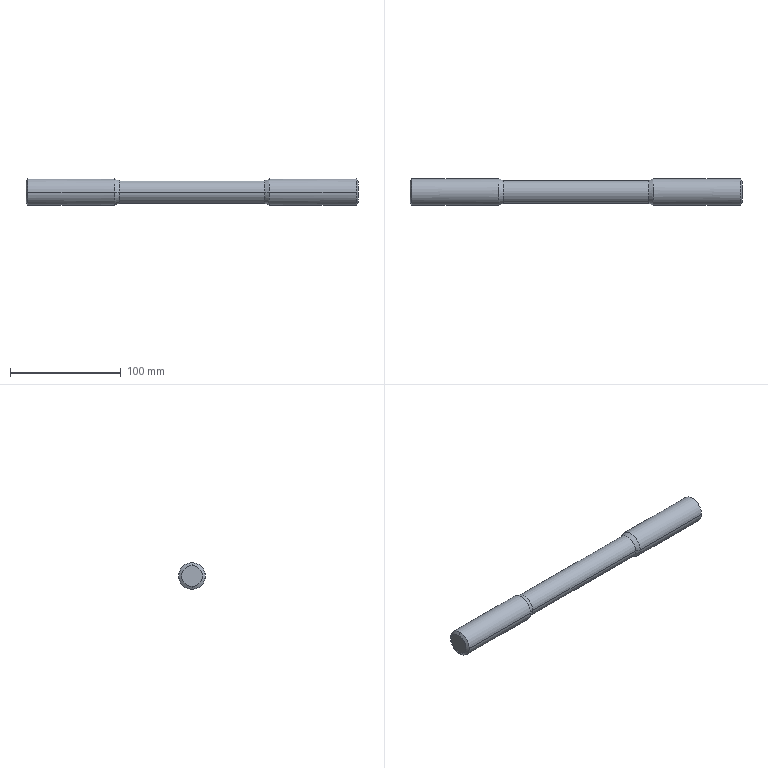Part | STEP file | GB/T901-1988 double-end stud, grade B, M24×300 | 1 solid | 16 faces | box 300 x 24 x 24 mm | volume 120071 mm3 | cone 8 | cylinder 6 | plane 2 | commonest cylinder face diameters 24 x4 20.784 x2
STEP:
#1=CARTESIAN_POINT('',(0.,0.,0.));
#2=DIRECTION('',(0.,0.,1.));
#3=DIRECTION('',(1.,0.,0.));
#4=AXIS2_PLACEMENT_3D('',#1,#2,#3);
#5=CARTESIAN_POINT('',(150.,0.,-9.402));
#6=VERTEX_POINT('',#5);
#7=CARTESIAN_POINT('',(150.,0.,9.402));
#8=VERTEX_POINT('',#7);
#9=CARTESIAN_POINT('',(150.,0.,0.));
#10=DIRECTION('',(-1.,0.,0.));
#11=DIRECTION('',(0.,0.,1.));
#12=AXIS2_PLACEMENT_3D('',#9,#10,#11);
#13=CIRCLE('',#12,9.402);
#14=CARTESIAN_POINT('',(150.,0.,0.));
#15=DIRECTION('',(-1.,0.,0.));
#16=DIRECTION('',(0.,0.,-1.));
#17=AXIS2_PLACEMENT_3D('',#14,#15,#16);
#18=CONICAL_SURFACE('',#17,9.402,1.047);
#19=CARTESIAN_POINT('',(-3.142,0.));
#20=DIRECTION('',(1.,0.));
#21=VECTOR('',#20,1.);
#22=LINE('',#19,#21);
#23=(GEOMETRIC_REPRESENTATION_CONTEXT(2)PARAMETRIC_REPRESENTATION_CONTEXT()REPRESENTATION_CONTEXT('',''));
#24=DEFINITIONAL_REPRESENTATION('',(#22),#23);
#25=PCURVE('',#18,#24);
#26=CARTESIAN_POINT('',(150.,12.,0.));
#27=DIRECTION('',(-1.,0.,0.));
#28=DIRECTION('',(0.,1.,0.));
#29=AXIS2_PLACEMENT_3D('',#26,#27,#28);
#30=PLANE('',#29);
#31=CARTESIAN_POINT('',(-12.,0.));
#32=DIRECTION('',(0.,-1.));
#33=AXIS2_PLACEMENT_2D('',#31,#32);
#34=CIRCLE('',#33,9.402);
#35=(GEOMETRIC_REPRESENTATION_CONTEXT(2)PARAMETRIC_REPRESENTATION_CONTEXT()REPRESENTATION_CONTEXT('',''));
#36=DEFINITIONAL_REPRESENTATION('',(#34),#35);
#37=PCURVE('',#30,#36);
#38=SURFACE_CURVE('',#13,(#25,#37),.PCURVE_S1.);
#39=EDGE_CURVE('',#6,#8,#38,.T.);
#40=ORIENTED_EDGE('',*,*,#39,.T.);
#41=CARTESIAN_POINT('',(148.5,0.,12.));
#42=VERTEX_POINT('',#41);
#43=CARTESIAN_POINT('',(150.,0.,9.402));
#44=DIRECTION('',(-0.5,0.,0.866));
#45=VECTOR('',#44,1.);
#46=LINE('',#43,#45);
#47=CARTESIAN_POINT('',(3.142,0.));
#48=DIRECTION('',(0.,1.));
#49=VECTOR('',#48,1.);
#50=LINE('',#47,#49);
#51=(GEOMETRIC_REPRESENTATION_CONTEXT(2)PARAMETRIC_REPRESENTATION_CONTEXT()REPRESENTATION_CONTEXT('',''));
#52=DEFINITIONAL_REPRESENTATION('',(#50),#51);
#53=PCURVE('',#18,#52);
#54=CARTESIAN_POINT('',(150.,0.,0.));
#55=DIRECTION('',(-1.,0.,0.));
#56=DIRECTION('',(0.,0.,-1.));
#57=AXIS2_PLACEMENT_3D('',#54,#55,#56);
#58=CONICAL_SURFACE('',#57,9.402,1.047);
#59=CARTESIAN_POINT('',(3.142,0.));
#60=DIRECTION('',(0.,1.));
#61=VECTOR('',#60,1.);
#62=LINE('',#59,#61);
#63=(GEOMETRIC_REPRESENTATION_CONTEXT(2)PARAMETRIC_REPRESENTATION_CONTEXT()REPRESENTATION_CONTEXT('',''));
#64=DEFINITIONAL_REPRESENTATION('',(#62),#63);
#65=PCURVE('',#58,#64);
#66=SURFACE_CURVE('',#46,(#53,#65),.PCURVE_S1.);
#67=EDGE_CURVE('',#8,#42,#66,.T.);
#68=ORIENTED_EDGE('',*,*,#67,.T.);
#69=CARTESIAN_POINT('',(148.5,-12.,0.));
#70=VERTEX_POINT('',#69);
#71=CARTESIAN_POINT('',(148.5,0.,0.));
#72=DIRECTION('',(-1.,0.,0.));
#73=DIRECTION('',(0.,0.,1.));
#74=AXIS2_PLACEMENT_3D('',#71,#72,#73);
#75=CIRCLE('',#74,12.);
#76=CARTESIAN_POINT('',(-3.142,1.5));
#77=DIRECTION('',(1.,0.));
#78=VECTOR('',#77,1.);
#79=LINE('',#76,#78);
#80=(GEOMETRIC_REPRESENTATION_CONTEXT(2)PARAMETRIC_REPRESENTATION_CONTEXT()REPRESENTATION_CONTEXT('',''));
#81=DEFINITIONAL_REPRESENTATION('',(#79),#80);
#82=PCURVE('',#18,#81);
#83=CARTESIAN_POINT('',(150.,0.,0.));
#84=DIRECTION('',(1.,0.,0.));
#85=DIRECTION('',(0.,-1.,0.));
#86=AXIS2_PLACEMENT_3D('',#83,#84,#85);
#87=CYLINDRICAL_SURFACE('',#86,12.);
#88=CARTESIAN_POINT('',(10.996,-1.5));
#89=DIRECTION('',(-1.,0.));
#90=VECTOR('',#89,1.);
#91=LINE('',#88,#90);
#92=(GEOMETRIC_REPRESENTATION_CONTEXT(2)PARAMETRIC_REPRESENTATION_CONTEXT()REPRESENTATION_CONTEXT('',''));
#93=DEFINITIONAL_REPRESENTATION('',(#91),#92);
#94=PCURVE('',#87,#93);
#95=SURFACE_CURVE('',#75,(#82,#94),.PCURVE_S1.);
#96=EDGE_CURVE('',#70,#42,#95,.T.);
#97=ORIENTED_EDGE('',*,*,#96,.F.);
#98=CARTESIAN_POINT('',(148.5,0.,-12.));
#99=VERTEX_POINT('',#98);
#100=CARTESIAN_POINT('',(148.5,0.,0.));
#101=DIRECTION('',(-1.,0.,0.));
#102=DIRECTION('',(0.,0.,1.));
#103=AXIS2_PLACEMENT_3D('',#100,#101,#102);
#104=CIRCLE('',#103,12.);
#105=CARTESIAN_POINT('',(-3.142,1.5));
#106=DIRECTION('',(1.,0.));
#107=VECTOR('',#106,1.);
#108=LINE('',#105,#107);
#109=(GEOMETRIC_REPRESENTATION_CONTEXT(2)PARAMETRIC_REPRESENTATION_CONTEXT()REPRESENTATION_CONTEXT('',''));
#110=DEFINITIONAL_REPRESENTATION('',(#108),#109);
#111=PCURVE('',#18,#110);
#112=CARTESIAN_POINT('',(150.,0.,0.));
#113=DIRECTION('',(1.,0.,0.));
#114=DIRECTION('',(0.,-1.,0.));
#115=AXIS2_PLACEMENT_3D('',#112,#113,#114);
#116=CYLINDRICAL_SURFACE('',#115,12.);
#117=CARTESIAN_POINT('',(4.712,-1.5));
#118=DIRECTION('',(-1.,0.));
#119=VECTOR('',#118,1.);
#120=LINE('',#117,#119);
#121=(GEOMETRIC_REPRESENTATION_CONTEXT(2)PARAMETRIC_REPRESENTATION_CONTEXT()REPRESENTATION_CONTEXT('',''));
#122=DEFINITIONAL_REPRESENTATION('',(#120),#121);
#123=PCURVE('',#116,#122);
#124=SURFACE_CURVE('',#104,(#111,#123),.PCURVE_S1.);
#125=EDGE_CURVE('',#99,#70,#124,.T.);
#126=ORIENTED_EDGE('',*,*,#125,.F.);
#127=CARTESIAN_POINT('',(150.,0.,-9.402));
#128=DIRECTION('',(-0.5,0.,-0.866));
#129=VECTOR('',#128,1.);
#130=LINE('',#127,#129);
#131=CARTESIAN_POINT('',(0.,0.));
#132=DIRECTION('',(0.,1.));
#133=VECTOR('',#132,1.);
#134=LINE('',#131,#133);
#135=(GEOMETRIC_REPRESENTATION_CONTEXT(2)PARAMETRIC_REPRESENTATION_CONTEXT()REPRESENTATION_CONTEXT('',''));
#136=DEFINITIONAL_REPRESENTATION('',(#134),#135);
#137=PCURVE('',#18,#136);
#138=CARTESIAN_POINT('',(6.283,0.));
#139=DIRECTION('',(0.,1.));
#140=VECTOR('',#139,1.);
#141=LINE('',#138,#140);
#142=(GEOMETRIC_REPRESENTATION_CONTEXT(2)PARAMETRIC_REPRESENTATION_CONTEXT()REPRESENTATION_CONTEXT('',''));
#143=DEFINITIONAL_REPRESENTATION('',(#141),#142);
#144=PCURVE('',#58,#143);
#145=SURFACE_CURVE('',#130,(#137,#144),.PCURVE_S1.);
#146=EDGE_CURVE('',#6,#99,#145,.T.);
#147=ORIENTED_EDGE('',*,*,#146,.F.);
#148=EDGE_LOOP('',(#40,#68,#97,#126,#147));
#149=FACE_BOUND('',#148,.T.);
#150=ADVANCED_FACE('',(#149),#18,.T.);
#151=CARTESIAN_POINT('',(65.8,10.392,0.));
#152=VERTEX_POINT('',#151);
#153=CARTESIAN_POINT('',(65.8,-10.392,0.));
#154=VERTEX_POINT('',#153);
#155=CARTESIAN_POINT('',(65.8,0.,0.));
#156=DIRECTION('',(-1.,0.,0.));
#157=DIRECTION('',(0.,-1.,0.));
#158=AXIS2_PLACEMENT_3D('',#155,#156,#157);
#159=CIRCLE('',#158,10.392);
#160=CARTESIAN_POINT('',(65.8,0.,0.));
#161=DIRECTION('',(1.,0.,0.));
#162=DIRECTION('',(0.,-1.,0.));
#163=AXIS2_PLACEMENT_3D('',#160,#161,#162);
#164=CONICAL_SURFACE('',#163,10.392,0.3656);
#165=CARTESIAN_POINT('',(6.283,0.));
#166=DIRECTION('',(-1.,0.));
#167=VECTOR('',#166,1.);
#168=LINE('',#165,#167);
#169=(GEOMETRIC_REPRESENTATION_CONTEXT(2)PARAMETRIC_REPRESENTATION_CONTEXT()REPRESENTATION_CONTEXT('',''));
#170=DEFINITIONAL_REPRESENTATION('',(#168),#169);
#171=PCURVE('',#164,#170);
#172=CARTESIAN_POINT('',(-150.,0.,0.));
#173=DIRECTION('',(-1.,0.,0.));
#174=DIRECTION('',(0.,-1.,0.));
#175=AXIS2_PLACEMENT_3D('',#172,#173,#174);
#176=CYLINDRICAL_SURFACE('',#175,10.392);
#177=CARTESIAN_POINT('',(0.,-215.8));
#178=DIRECTION('',(1.,0.));
#179=VECTOR('',#178,1.);
#180=LINE('',#177,#179);
#181=(GEOMETRIC_REPRESENTATION_CONTEXT(2)PARAMETRIC_REPRESENTATION_CONTEXT()REPRESENTATION_CONTEXT('',''));
#182=DEFINITIONAL_REPRESENTATION('',(#180),#181);
#183=PCURVE('',#176,#182);
#184=SURFACE_CURVE('',#159,(#171,#183),.PCURVE_S1.);
#185=EDGE_CURVE('',#152,#154,#184,.T.);
#186=ORIENTED_EDGE('',*,*,#185,.F.);
#187=CARTESIAN_POINT('',(70.,12.,0.));
#188=VERTEX_POINT('',#187);
#189=CARTESIAN_POINT('',(65.8,10.392,0.));
#190=DIRECTION('',(0.9339,0.3575,0.));
#191=VECTOR('',#190,1.);
#192=LINE('',#189,#191);
#193=CARTESIAN_POINT('',(3.142,0.));
#194=DIRECTION('',(0.,1.));
#195=VECTOR('',#194,1.);
#196=LINE('',#193,#195);
#197=(GEOMETRIC_REPRESENTATION_CONTEXT(2)PARAMETRIC_REPRESENTATION_CONTEXT()REPRESENTATION_CONTEXT('',''));
#198=DEFINITIONAL_REPRESENTATION('',(#196),#197);
#199=PCURVE('',#164,#198);
#200=CARTESIAN_POINT('',(65.8,0.,0.));
#201=DIRECTION('',(1.,0.,0.));
#202=DIRECTION('',(0.,-1.,0.));
#203=AXIS2_PLACEMENT_3D('',#200,#201,#202);
#204=CONICAL_SURFACE('',#203,10.392,0.3656);
#205=CARTESIAN_POINT('',(3.142,0.));
#206=DIRECTION('',(0.,1.));
#207=VECTOR('',#206,1.);
#208=LINE('',#205,#207);
#209=(GEOMETRIC_REPRESENTATION_CONTEXT(2)PARAMETRIC_REPRESENTATION_CONTEXT()REPRESENTATION_CONTEXT('',''));
#210=DEFINITIONAL_REPRESENTATION('',(#208),#209);
#211=PCURVE('',#204,#210);
#212=SURFACE_CURVE('',#192,(#199,#211),.PCURVE_S1.);
#213=EDGE_CURVE('',#152,#188,#212,.T.);
#214=ORIENTED_EDGE('',*,*,#213,.T.);
#215=CARTESIAN_POINT('',(70.,-12.,0.));
#216=VERTEX_POINT('',#215);
#217=CARTESIAN_POINT('',(70.,0.,0.));
#218=DIRECTION('',(-1.,0.,0.));
#219=DIRECTION('',(0.,-1.,0.));
#220=AXIS2_PLACEMENT_3D('',#217,#218,#219);
#221=CIRCLE('',#220,12.);
#222=CARTESIAN_POINT('',(6.283,4.2));
#223=DIRECTION('',(-1.,0.));
#224=VECTOR('',#223,1.);
#225=LINE('',#222,#224);
#226=(GEOMETRIC_REPRESENTATION_CONTEXT(2)PARAMETRIC_REPRESENTATION_CONTEXT()REPRESENTATION_CONTEXT('',''));
#227=DEFINITIONAL_REPRESENTATION('',(#225),#226);
#228=PCURVE('',#164,#227);
#229=CARTESIAN_POINT('',(6.283,-80.));
#230=DIRECTION('',(-1.,0.));
#231=VECTOR('',#230,1.);
#232=LINE('',#229,#231);
#233=(GEOMETRIC_REPRESENTATION_CONTEXT(2)PARAMETRIC_REPRESENTATION_CONTEXT()REPRESENTATION_CONTEXT('',''));
#234=DEFINITIONAL_REPRESENTATION('',(#232),#233);
#235=PCURVE('',#116,#234);
#236=SURFACE_CURVE('',#221,(#228,#235),.PCURVE_S1.);
#237=EDGE_CURVE('',#188,#216,#236,.T.);
#238=ORIENTED_EDGE('',*,*,#237,.T.);
#239=CARTESIAN_POINT('',(65.8,-10.392,0.));
#240=DIRECTION('',(0.9339,-0.3575,0.));
#241=VECTOR('',#240,1.);
#242=LINE('',#239,#241);
#243=CARTESIAN_POINT('',(0.,0.));
#244=DIRECTION('',(0.,1.));
#245=VECTOR('',#244,1.);
#246=LINE('',#243,#245);
#247=(GEOMETRIC_REPRESENTATION_CONTEXT(2)PARAMETRIC_REPRESENTATION_CONTEXT()REPRESENTATION_CONTEXT('',''));
#248=DEFINITIONAL_REPRESENTATION('',(#246),#247);
#249=PCURVE('',#164,#248);
#250=CARTESIAN_POINT('',(6.283,0.));
#251=DIRECTION('',(0.,1.));
#252=VECTOR('',#251,1.);
#253=LINE('',#250,#252);
#254=(GEOMETRIC_REPRESENTATION_CONTEXT(2)PARAMETRIC_REPRESENTATION_CONTEXT()REPRESENTATION_CONTEXT('',''));
#255=DEFINITIONAL_REPRESENTATION('',(#253),#254);
#256=PCURVE('',#204,#255);
#257=SURFACE_CURVE('',#242,(#249,#256),.PCURVE_S1.);
#258=EDGE_CURVE('',#154,#216,#257,.T.);
#259=ORIENTED_EDGE('',*,*,#258,.F.);
#260=EDGE_LOOP('',(#186,#214,#238,#259));
#261=FACE_BOUND('',#260,.T.);
#262=ADVANCED_FACE('',(#261),#164,.T.);
#263=ORIENTED_EDGE('',*,*,#237,.F.);
#264=CARTESIAN_POINT('',(148.5,12.,0.));
#265=VERTEX_POINT('',#264);
#266=CARTESIAN_POINT('',(150.,12.,0.));
#267=DIRECTION('',(1.,0.,0.));
#268=VECTOR('',#267,1.);
#269=LINE('',#266,#268);
#270=CARTESIAN_POINT('',(3.142,0.));
#271=DIRECTION('',(0.,1.));
#272=VECTOR('',#271,1.);
#273=LINE('',#270,#272);
#274=(GEOMETRIC_REPRESENTATION_CONTEXT(2)PARAMETRIC_REPRESENTATION_CONTEXT()REPRESENTATION_CONTEXT('',''));
#275=DEFINITIONAL_REPRESENTATION('',(#273),#274);
#276=PCURVE('',#116,#275);
#277=CARTESIAN_POINT('',(3.142,0.));
#278=DIRECTION('',(0.,1.));
#279=VECTOR('',#278,1.);
#280=LINE('',#277,#279);
#281=(GEOMETRIC_REPRESENTATION_CONTEXT(2)PARAMETRIC_REPRESENTATION_CONTEXT()REPRESENTATION_CONTEXT('',''));
#282=DEFINITIONAL_REPRESENTATION('',(#280),#281);
#283=PCURVE('',#87,#282);
#284=SURFACE_CURVE('',#269,(#276,#283),.PCURVE_S1.);
#285=EDGE_CURVE('',#188,#265,#284,.T.);
#286=ORIENTED_EDGE('',*,*,#285,.T.);
#287=CARTESIAN_POINT('',(148.5,0.,0.));
#288=DIRECTION('',(-1.,0.,0.));
#289=DIRECTION('',(0.,0.,1.));
#290=AXIS2_PLACEMENT_3D('',#287,#288,#289);
#291=CIRCLE('',#290,12.);
#292=CARTESIAN_POINT('',(4.712,-1.5));
#293=DIRECTION('',(-1.,0.));
#294=VECTOR('',#293,1.);
#295=LINE('',#292,#294);
#296=(GEOMETRIC_REPRESENTATION_CONTEXT(2)PARAMETRIC_REPRESENTATION_CONTEXT()REPRESENTATION_CONTEXT('',''));
#297=DEFINITIONAL_REPRESENTATION('',(#295),#296);
#298=PCURVE('',#116,#297);
#299=CARTESIAN_POINT('',(3.142,1.5));
#300=DIRECTION('',(1.,0.));
#301=VECTOR('',#300,1.);
#302=LINE('',#299,#301);
#303=(GEOMETRIC_REPRESENTATION_CONTEXT(2)PARAMETRIC_REPRESENTATION_CONTEXT()REPRESENTATION_CONTEXT('',''));
#304=DEFINITIONAL_REPRESENTATION('',(#302),#303);
#305=PCURVE('',#58,#304);
#306=SURFACE_CURVE('',#291,(#298,#305),.PCURVE_S1.);
#307=EDGE_CURVE('',#265,#99,#306,.T.);
#308=ORIENTED_EDGE('',*,*,#307,.T.);
#309=ORIENTED_EDGE('',*,*,#125,.T.);
#310=CARTESIAN_POINT('',(150.,-12.,0.));
#311=DIRECTION('',(1.,0.,0.));
#312=VECTOR('',#311,1.);
#313=LINE('',#310,#312);
#314=CARTESIAN_POINT('',(0.,0.));
#315=DIRECTION('',(0.,1.));
#316=VECTOR('',#315,1.);
#317=LINE('',#314,#316);
#318=(GEOMETRIC_REPRESENTATION_CONTEXT(2)PARAMETRIC_REPRESENTATION_CONTEXT()REPRESENTATION_CONTEXT('',''));
#319=DEFINITIONAL_REPRESENTATION('',(#317),#318);
#320=PCURVE('',#116,#319);
#321=CARTESIAN_POINT('',(6.283,0.));
#322=DIRECTION('',(0.,1.));
#323=VECTOR('',#322,1.);
#324=LINE('',#321,#323);
#325=(GEOMETRIC_REPRESENTATION_CONTEXT(2)PARAMETRIC_REPRESENTATION_CONTEXT()REPRESENTATION_CONTEXT('',''));
#326=DEFINITIONAL_REPRESENTATION('',(#324),#325);
#327=PCURVE('',#87,#326);
#328=SURFACE_CURVE('',#313,(#320,#327),.PCURVE_S1.);
#329=EDGE_CURVE('',#216,#70,#328,.T.);
#330=ORIENTED_EDGE('',*,*,#329,.F.);
#331=EDGE_LOOP('',(#263,#286,#308,#309,#330));
#332=FACE_BOUND('',#331,.T.);
#333=ADVANCED_FACE('',(#332),#116,.T.);
#334=CARTESIAN_POINT('',(-150.,0.,9.402));
#335=VERTEX_POINT('',#334);
#336=CARTESIAN_POINT('',(-150.,0.,-9.402));
#337=VERTEX_POINT('',#336);
#338=CARTESIAN_POINT('',(-150.,0.,0.));
#339=DIRECTION('',(-1.,0.,0.));
#340=DIRECTION('',(0.,0.,1.));
#341=AXIS2_PLACEMENT_3D('',#338,#339,#340);
#342=CIRCLE('',#341,9.402);
#343=CARTESIAN_POINT('',(-150.,0.,0.));
#344=DIRECTION('',(1.,0.,0.));
#345=DIRECTION('',(0.,0.,-1.));
#346=AXIS2_PLACEMENT_3D('',#343,#344,#345);
#347=CONICAL_SURFACE('',#346,9.402,1.047);
#348=CARTESIAN_POINT('',(3.142,0.));
#349=DIRECTION('',(-1.,0.));
#350=VECTOR('',#349,1.);
#351=LINE('',#348,#350);
#352=(GEOMETRIC_REPRESENTATION_CONTEXT(2)PARAMETRIC_REPRESENTATION_CONTEXT()REPRESENTATION_CONTEXT('',''));
#353=DEFINITIONAL_REPRESENTATION('',(#351),#352);
#354=PCURVE('',#347,#353);
#355=CARTESIAN_POINT('',(-150.,12.,0.));
#356=DIRECTION('',(1.,0.,0.));
#357=DIRECTION('',(0.,1.,0.));
#358=AXIS2_PLACEMENT_3D('',#355,#356,#357);
#359=PLANE('',#358);
#360=CARTESIAN_POINT('',(-12.,9.402));
#361=CARTESIAN_POINT('',(4.285,9.402));
#362=CARTESIAN_POINT('',(-3.858,-4.701));
#363=CARTESIAN_POINT('',(-12.,-18.804));
#364=CARTESIAN_POINT('',(-20.142,-4.701));
#365=CARTESIAN_POINT('',(-28.285,9.402));
#366=CARTESIAN_POINT('',(-12.,9.402));
#367=(BOUNDED_CURVE()B_SPLINE_CURVE(2,(#360,#361,#362,#363,#364,#365,#366),.UNSPECIFIED.,.T.,.F.)B_SPLINE_CURVE_WITH_KNOTS((1,2,2,2,2,1),(-2.094,0.,2.094,4.189,6.283,8.378),.UNSPECIFIED.)CURVE()GEOMETRIC_REPRESENTATION_ITEM()RATIONAL_B_SPLINE_CURVE((1.,0.5,1.,0.5,1.,0.5,1.))REPRESENTATION_ITEM(''));
#368=(GEOMETRIC_REPRESENTATION_CONTEXT(2)PARAMETRIC_REPRESENTATION_CONTEXT()REPRESENTATION_CONTEXT('',''));
#369=DEFINITIONAL_REPRESENTATION('',(#367),#368);
#370=PCURVE('',#359,#369);
#371=SURFACE_CURVE('',#342,(#354,#370),.PCURVE_S1.);
#372=EDGE_CURVE('',#335,#337,#371,.T.);
#373=ORIENTED_EDGE('',*,*,#372,.F.);
#374=CARTESIAN_POINT('',(-148.5,0.,12.));
#375=VERTEX_POINT('',#374);
#376=CARTESIAN_POINT('',(-150.,0.,9.402));
#377=DIRECTION('',(0.5,0.,0.866));
#378=VECTOR('',#377,1.);
#379=LINE('',#376,#378);
#380=CARTESIAN_POINT('',(3.142,0.));
#381=DIRECTION('',(0.,1.));
#382=VECTOR('',#381,1.);
#383=LINE('',#380,#382);
#384=(GEOMETRIC_REPRESENTATION_CONTEXT(2)PARAMETRIC_REPRESENTATION_CONTEXT()REPRESENTATION_CONTEXT('',''));
#385=DEFINITIONAL_REPRESENTATION('',(#383),#384);
#386=PCURVE('',#347,#385);
#387=CARTESIAN_POINT('',(-150.,0.,0.));
#388=DIRECTION('',(1.,0.,0.));
#389=DIRECTION('',(0.,0.,-1.));
#390=AXIS2_PLACEMENT_3D('',#387,#388,#389);
#391=CONICAL_SURFACE('',#390,9.402,1.047);
#392=CARTESIAN_POINT('',(3.142,0.));
#393=DIRECTION('',(0.,1.));
#394=VECTOR('',#393,1.);
#395=LINE('',#392,#394);
#396=(GEOMETRIC_REPRESENTATION_CONTEXT(2)PARAMETRIC_REPRESENTATION_CONTEXT()REPRESENTATION_CONTEXT('',''));
#397=DEFINITIONAL_REPRESENTATION('',(#395),#396);
#398=PCURVE('',#391,#397);
#399=SURFACE_CURVE('',#379,(#386,#398),.PCURVE_S1.);
#400=EDGE_CURVE('',#335,#375,#399,.T.);
#401=ORIENTED_EDGE('',*,*,#400,.T.);
#402=CARTESIAN_POINT('',(-148.5,12.,0.));
#403=VERTEX_POINT('',#402);
#404=CARTESIAN_POINT('',(-148.5,0.,0.));
#405=DIRECTION('',(-1.,0.,0.));
#406=DIRECTION('',(0.,0.,1.));
#407=AXIS2_PLACEMENT_3D('',#404,#405,#406);
#408=CIRCLE('',#407,12.);
#409=CARTESIAN_POINT('',(3.142,1.5));
#410=DIRECTION('',(-1.,0.));
#411=VECTOR('',#410,1.);
#412=LINE('',#409,#411);
#413=(GEOMETRIC_REPRESENTATION_CONTEXT(2)PARAMETRIC_REPRESENTATION_CONTEXT()REPRESENTATION_CONTEXT('',''));
#414=DEFINITIONAL_REPRESENTATION('',(#412),#413);
#415=PCURVE('',#347,#414);
#416=CARTESIAN_POINT('',(-150.,0.,0.));
#417=DIRECTION('',(-1.,0.,0.));
#418=DIRECTION('',(0.,-1.,0.));
#419=AXIS2_PLACEMENT_3D('',#416,#417,#418);
#420=CYLINDRICAL_SURFACE('',#419,12.);
#421=CARTESIAN_POINT('',(1.571,-1.5));
#422=DIRECTION('',(1.,0.));
#423=VECTOR('',#422,1.);
#424=LINE('',#421,#423);
#425=(GEOMETRIC_REPRESENTATION_CONTEXT(2)PARAMETRIC_REPRESENTATION_CONTEXT()REPRESENTATION_CONTEXT('',''));
#426=DEFINITIONAL_REPRESENTATION('',(#424),#425);
#427=PCURVE('',#420,#426);
#428=SURFACE_CURVE('',#408,(#415,#427),.PCURVE_S1.);
#429=EDGE_CURVE('',#375,#403,#428,.T.);
#430=ORIENTED_EDGE('',*,*,#429,.T.);
#431=CARTESIAN_POINT('',(-148.5,0.,-12.));
#432=VERTEX_POINT('',#431);
#433=CARTESIAN_POINT('',(-148.5,0.,0.));
#434=DIRECTION('',(-1.,0.,0.));
#435=DIRECTION('',(0.,0.,1.));
#436=AXIS2_PLACEMENT_3D('',#433,#434,#435);
#437=CIRCLE('',#436,12.);
#438=CARTESIAN_POINT('',(3.142,1.5));
#439=DIRECTION('',(-1.,0.));
#440=VECTOR('',#439,1.);
#441=LINE('',#438,#440);
#442=(GEOMETRIC_REPRESENTATION_CONTEXT(2)PARAMETRIC_REPRESENTATION_CONTEXT()REPRESENTATION_CONTEXT('',''));
#443=DEFINITIONAL_REPRESENTATION('',(#441),#442);
#444=PCURVE('',#347,#443);
#445=CARTESIAN_POINT('',(-150.,0.,0.));
#446=DIRECTION('',(-1.,0.,0.));
#447=DIRECTION('',(0.,-1.,0.));
#448=AXIS2_PLACEMENT_3D('',#445,#446,#447);
#449=CYLINDRICAL_SURFACE('',#448,12.);
#450=CARTESIAN_POINT('',(1.571,-1.5));
#451=DIRECTION('',(1.,0.));
#452=VECTOR('',#451,1.);
#453=LINE('',#450,#452);
#454=(GEOMETRIC_REPRESENTATION_CONTEXT(2)PARAMETRIC_REPRESENTATION_CONTEXT()REPRESENTATION_CONTEXT('',''));
#455=DEFINITIONAL_REPRESENTATION('',(#453),#454);
#456=PCURVE('',#449,#455);
#457=SURFACE_CURVE('',#437,(#444,#456),.PCURVE_S1.);
#458=EDGE_CURVE('',#403,#432,#457,.T.);
#459=ORIENTED_EDGE('',*,*,#458,.T.);
#460=CARTESIAN_POINT('',(-150.,0.,-9.402));
#461=DIRECTION('',(0.5,0.,-0.866));
#462=VECTOR('',#461,1.);
#463=LINE('',#460,#462);
#464=CARTESIAN_POINT('',(0.,0.));
#465=DIRECTION('',(0.,1.));
#466=VECTOR('',#465,1.);
#467=LINE('',#464,#466);
#468=(GEOMETRIC_REPRESENTATION_CONTEXT(2)PARAMETRIC_REPRESENTATION_CONTEXT()REPRESENTATION_CONTEXT('',''));
#469=DEFINITIONAL_REPRESENTATION('',(#467),#468);
#470=PCURVE('',#347,#469);
#471=CARTESIAN_POINT('',(6.283,0.));
#472=DIRECTION('',(0.,1.));
#473=VECTOR('',#472,1.);
#474=LINE('',#471,#473);
#475=(GEOMETRIC_REPRESENTATION_CONTEXT(2)PARAMETRIC_REPRESENTATION_CONTEXT()REPRESENTATION_CONTEXT('',''));
#476=DEFINITIONAL_REPRESENTATION('',(#474),#475);
#477=PCURVE('',#391,#476);
#478=SURFACE_CURVE('',#463,(#470,#477),.PCURVE_S1.);
#479=EDGE_CURVE('',#337,#432,#478,.T.);
#480=ORIENTED_EDGE('',*,*,#479,.F.);
#481=EDGE_LOOP('',(#373,#401,#430,#459,#480));
#482=FACE_BOUND('',#481,.T.);
#483=ADVANCED_FACE('',(#482),#347,.T.);
#484=CARTESIAN_POINT('',(-65.8,-10.392,0.));
#485=VERTEX_POINT('',#484);
#486=CARTESIAN_POINT('',(-65.8,10.392,0.));
#487=VERTEX_POINT('',#486);
#488=CARTESIAN_POINT('',(-65.8,0.,0.));
#489=DIRECTION('',(-1.,0.,0.));
#490=DIRECTION('',(0.,-1.,0.));
#491=AXIS2_PLACEMENT_3D('',#488,#489,#490);
#492=CIRCLE('',#491,10.392);
#493=CARTESIAN_POINT('',(-65.8,0.,0.));
#494=DIRECTION('',(-1.,0.,0.));
#495=DIRECTION('',(0.,-1.,0.));
#496=AXIS2_PLACEMENT_3D('',#493,#494,#495);
#497=CONICAL_SURFACE('',#496,10.392,0.3656);
#498=CARTESIAN_POINT('',(0.,0.));
#499=DIRECTION('',(1.,0.));
#500=VECTOR('',#499,1.);
#501=LINE('',#498,#500);
#502=(GEOMETRIC_REPRESENTATION_CONTEXT(2)PARAMETRIC_REPRESENTATION_CONTEXT()REPRESENTATION_CONTEXT('',''));
#503=DEFINITIONAL_REPRESENTATION('',(#501),#502);
#504=PCURVE('',#497,#503);
#505=CARTESIAN_POINT('',(-150.,0.,0.));
#506=DIRECTION('',(-1.,0.,0.));
#507=DIRECTION('',(0.,-1.,0.));
#508=AXIS2_PLACEMENT_3D('',#505,#506,#507);
#509=CYLINDRICAL_SURFACE('',#508,10.392);
#510=CARTESIAN_POINT('',(0.,-84.2));
#511=DIRECTION('',(1.,0.));
#512=VECTOR('',#511,1.);
#513=LINE('',#510,#512);
#514=(GEOMETRIC_REPRESENTATION_CONTEXT(2)PARAMETRIC_REPRESENTATION_CONTEXT()REPRESENTATION_CONTEXT('',''));
#515=DEFINITIONAL_REPRESENTATION('',(#513),#514);
#516=PCURVE('',#509,#515);
#517=SURFACE_CURVE('',#492,(#504,#516),.PCURVE_S1.);
#518=EDGE_CURVE('',#485,#487,#517,.T.);
#519=ORIENTED_EDGE('',*,*,#518,.T.);
#520=CARTESIAN_POINT('',(-70.,12.,0.));
#521=VERTEX_POINT('',#520);
#522=CARTESIAN_POINT('',(-65.8,10.392,0.));
#523=DIRECTION('',(-0.9339,0.3575,0.));
#524=VECTOR('',#523,1.);
#525=LINE('',#522,#524);
#526=CARTESIAN_POINT('',(3.142,0.));
#527=DIRECTION('',(0.,1.));
#528=VECTOR('',#527,1.);
#529=LINE('',#526,#528);
#530=(GEOMETRIC_REPRESENTATION_CONTEXT(2)PARAMETRIC_REPRESENTATION_CONTEXT()REPRESENTATION_CONTEXT('',''));
#531=DEFINITIONAL_REPRESENTATION('',(#529),#530);
#532=PCURVE('',#497,#531);
#533=CARTESIAN_POINT('',(-65.8,0.,0.));
#534=DIRECTION('',(-1.,0.,0.));
#535=DIRECTION('',(0.,-1.,0.));
#536=AXIS2_PLACEMENT_3D('',#533,#534,#535);
#537=CONICAL_SURFACE('',#536,10.392,0.3656);
#538=CARTESIAN_POINT('',(3.142,0.));
#539=DIRECTION('',(0.,1.));
#540=VECTOR('',#539,1.);
#541=LINE('',#538,#540);
#542=(GEOMETRIC_REPRESENTATION_CONTEXT(2)PARAMETRIC_REPRESENTATION_CONTEXT()REPRESENTATION_CONTEXT('',''));
#543=DEFINITIONAL_REPRESENTATION('',(#541),#542);
#544=PCURVE('',#537,#543);
#545=SURFACE_CURVE('',#525,(#532,#544),.PCURVE_S1.);
#546=EDGE_CURVE('',#487,#521,#545,.T.);
#547=ORIENTED_EDGE('',*,*,#546,.T.);
#548=CARTESIAN_POINT('',(-70.,-12.,0.));
#549=VERTEX_POINT('',#548);
#550=CARTESIAN_POINT('',(-70.,0.,0.));
#551=DIRECTION('',(-1.,0.,0.));
#552=DIRECTION('',(0.,-1.,0.));
#553=AXIS2_PLACEMENT_3D('',#550,#551,#552);
#554=CIRCLE('',#553,12.);
#555=CARTESIAN_POINT('',(0.,4.2));
#556=DIRECTION('',(1.,0.));
#557=VECTOR('',#556,1.);
#558=LINE('',#555,#557);
#559=(GEOMETRIC_REPRESENTATION_CONTEXT(2)PARAMETRIC_REPRESENTATION_CONTEXT()REPRESENTATION_CONTEXT('',''));
#560=DEFINITIONAL_REPRESENTATION('',(#558),#559);
#561=PCURVE('',#497,#560);
#562=CARTESIAN_POINT('',(0.,-80.));
#563=DIRECTION('',(1.,0.));
#564=VECTOR('',#563,1.);
#565=LINE('',#562,#564);
#566=(GEOMETRIC_REPRESENTATION_CONTEXT(2)PARAMETRIC_REPRESENTATION_CONTEXT()REPRESENTATION_CONTEXT('',''));
#567=DEFINITIONAL_REPRESENTATION('',(#565),#566);
#568=PCURVE('',#420,#567);
#569=SURFACE_CURVE('',#554,(#561,#568),.PCURVE_S1.);
#570=EDGE_CURVE('',#549,#521,#569,.T.);
#571=ORIENTED_EDGE('',*,*,#570,.F.);
#572=CARTESIAN_POINT('',(-65.8,-10.392,0.));
#573=DIRECTION('',(-0.9339,-0.3575,0.));
#574=VECTOR('',#573,1.);
#575=LINE('',#572,#574);
#576=CARTESIAN_POINT('',(0.,0.));
#577=DIRECTION('',(0.,1.));
#578=VECTOR('',#577,1.);
#579=LINE('',#576,#578);
#580=(GEOMETRIC_REPRESENTATION_CONTEXT(2)PARAMETRIC_REPRESENTATION_CONTEXT()REPRESENTATION_CONTEXT('',''));
#581=DEFINITIONAL_REPRESENTATION('',(#579),#580);
#582=PCURVE('',#497,#581);
#583=CARTESIAN_POINT('',(6.283,0.));
#584=DIRECTION('',(0.,1.));
#585=VECTOR('',#584,1.);
#586=LINE('',#583,#585);
#587=(GEOMETRIC_REPRESENTATION_CONTEXT(2)PARAMETRIC_REPRESENTATION_CONTEXT()REPRESENTATION_CONTEXT('',''));
#588=DEFINITIONAL_REPRESENTATION('',(#586),#587);
#589=PCURVE('',#537,#588);
#590=SURFACE_CURVE('',#575,(#582,#589),.PCURVE_S1.);
#591=EDGE_CURVE('',#485,#549,#590,.T.);
#592=ORIENTED_EDGE('',*,*,#591,.F.);
#593=EDGE_LOOP('',(#519,#547,#571,#592));
#594=FACE_BOUND('',#593,.T.);
#595=ADVANCED_FACE('',(#594),#497,.T.);
#596=CARTESIAN_POINT('',(65.8,0.,0.));
#597=DIRECTION('',(-1.,0.,0.));
#598=DIRECTION('',(0.,-1.,0.));
#599=AXIS2_PLACEMENT_3D('',#596,#597,#598);
#600=CIRCLE('',#599,10.392);
#601=CARTESIAN_POINT('',(0.,-215.8));
#602=DIRECTION('',(1.,0.));
#603=VECTOR('',#602,1.);
#604=LINE('',#601,#603);
#605=(GEOMETRIC_REPRESENTATION_CONTEXT(2)PARAMETRIC_REPRESENTATION_CONTEXT()REPRESENTATION_CONTEXT('',''));
#606=DEFINITIONAL_REPRESENTATION('',(#604),#605);
#607=PCURVE('',#509,#606);
#608=CARTESIAN_POINT('',(6.283,0.));
#609=DIRECTION('',(-1.,0.));
#610=VECTOR('',#609,1.);
#611=LINE('',#608,#610);
#612=(GEOMETRIC_REPRESENTATION_CONTEXT(2)PARAMETRIC_REPRESENTATION_CONTEXT()REPRESENTATION_CONTEXT('',''));
#613=DEFINITIONAL_REPRESENTATION('',(#611),#612);
#614=PCURVE('',#204,#613);
#615=SURFACE_CURVE('',#600,(#607,#614),.PCURVE_S1.);
#616=EDGE_CURVE('',#154,#152,#615,.T.);
#617=ORIENTED_EDGE('',*,*,#616,.T.);
#618=CARTESIAN_POINT('',(-150.,10.392,0.));
#619=DIRECTION('',(-1.,0.,0.));
#620=VECTOR('',#619,1.);
#621=LINE('',#618,#620);
#622=CARTESIAN_POINT('',(3.142,0.));
#623=DIRECTION('',(0.,1.));
#624=VECTOR('',#623,1.);
#625=LINE('',#622,#624);
#626=(GEOMETRIC_REPRESENTATION_CONTEXT(2)PARAMETRIC_REPRESENTATION_CONTEXT()REPRESENTATION_CONTEXT('',''));
#627=DEFINITIONAL_REPRESENTATION('',(#625),#626);
#628=PCURVE('',#509,#627);
#629=CARTESIAN_POINT('',(3.142,0.));
#630=DIRECTION('',(0.,1.));
#631=VECTOR('',#630,1.);
#632=LINE('',#629,#631);
#633=(GEOMETRIC_REPRESENTATION_CONTEXT(2)PARAMETRIC_REPRESENTATION_CONTEXT()REPRESENTATION_CONTEXT('',''));
#634=DEFINITIONAL_REPRESENTATION('',(#632),#633);
#635=PCURVE('',#176,#634);
#636=SURFACE_CURVE('',#621,(#628,#635),.PCURVE_S1.);
#637=EDGE_CURVE('',#152,#487,#636,.T.);
#638=ORIENTED_EDGE('',*,*,#637,.T.);
#639=ORIENTED_EDGE('',*,*,#518,.F.);
#640=CARTESIAN_POINT('',(-150.,-10.392,0.));
#641=DIRECTION('',(-1.,0.,0.));
#642=VECTOR('',#641,1.);
#643=LINE('',#640,#642);
#644=CARTESIAN_POINT('',(0.,0.));
#645=DIRECTION('',(0.,1.));
#646=VECTOR('',#645,1.);
#647=LINE('',#644,#646);
#648=(GEOMETRIC_REPRESENTATION_CONTEXT(2)PARAMETRIC_REPRESENTATION_CONTEXT()REPRESENTATION_CONTEXT('',''));
#649=DEFINITIONAL_REPRESENTATION('',(#647),#648);
#650=PCURVE('',#509,#649);
#651=CARTESIAN_POINT('',(6.283,0.));
#652=DIRECTION('',(0.,1.));
#653=VECTOR('',#652,1.);
#654=LINE('',#651,#653);
#655=(GEOMETRIC_REPRESENTATION_CONTEXT(2)PARAMETRIC_REPRESENTATION_CONTEXT()REPRESENTATION_CONTEXT('',''));
#656=DEFINITIONAL_REPRESENTATION('',(#654),#655);
#657=PCURVE('',#176,#656);
#658=SURFACE_CURVE('',#643,(#650,#657),.PCURVE_S1.);
#659=EDGE_CURVE('',#154,#485,#658,.T.);
#660=ORIENTED_EDGE('',*,*,#659,.F.);
#661=EDGE_LOOP('',(#617,#638,#639,#660));
#662=FACE_BOUND('',#661,.T.);
#663=ADVANCED_FACE('',(#662),#509,.T.);
#664=ORIENTED_EDGE('',*,*,#570,.T.);
#665=CARTESIAN_POINT('',(-150.,12.,0.));
#666=DIRECTION('',(-1.,0.,0.));
#667=VECTOR('',#666,1.);
#668=LINE('',#665,#667);
#669=CARTESIAN_POINT('',(3.142,0.));
#670=DIRECTION('',(0.,1.));
#671=VECTOR('',#670,1.);
#672=LINE('',#669,#671);
#673=(GEOMETRIC_REPRESENTATION_CONTEXT(2)PARAMETRIC_REPRESENTATION_CONTEXT()REPRESENTATION_CONTEXT('',''));
#674=DEFINITIONAL_REPRESENTATION('',(#672),#673);
#675=PCURVE('',#420,#674);
#676=CARTESIAN_POINT('',(3.142,0.));
#677=DIRECTION('',(0.,1.));
#678=VECTOR('',#677,1.);
#679=LINE('',#676,#678);
#680=(GEOMETRIC_REPRESENTATION_CONTEXT(2)PARAMETRIC_REPRESENTATION_CONTEXT()REPRESENTATION_CONTEXT('',''));
#681=DEFINITIONAL_REPRESENTATION('',(#679),#680);
#682=PCURVE('',#449,#681);
#683=SURFACE_CURVE('',#668,(#675,#682),.PCURVE_S1.);
#684=EDGE_CURVE('',#521,#403,#683,.T.);
#685=ORIENTED_EDGE('',*,*,#684,.T.);
#686=ORIENTED_EDGE('',*,*,#429,.F.);
#687=CARTESIAN_POINT('',(-148.5,-12.,0.));
#688=VERTEX_POINT('',#687);
#689=CARTESIAN_POINT('',(-148.5,0.,0.));
#690=DIRECTION('',(-1.,0.,0.));
#691=DIRECTION('',(0.,0.,1.));
#692=AXIS2_PLACEMENT_3D('',#689,#690,#691);
#693=CIRCLE('',#692,12.);
#694=CARTESIAN_POINT('',(-4.712,-1.5));
#695=DIRECTION('',(1.,0.));
#696=VECTOR('',#695,1.);
#697=LINE('',#694,#696);
#698=(GEOMETRIC_REPRESENTATION_CONTEXT(2)PARAMETRIC_REPRESENTATION_CONTEXT()REPRESENTATION_CONTEXT('',''));
#699=DEFINITIONAL_REPRESENTATION('',(#697),#698);
#700=PCURVE('',#420,#699);
#701=CARTESIAN_POINT('',(9.425,1.5));
#702=DIRECTION('',(-1.,0.));
#703=VECTOR('',#702,1.);
#704=LINE('',#701,#703);
#705=(GEOMETRIC_REPRESENTATION_CONTEXT(2)PARAMETRIC_REPRESENTATION_CONTEXT()REPRESENTATION_CONTEXT('',''));
#706=DEFINITIONAL_REPRESENTATION('',(#704),#705);
#707=PCURVE('',#391,#706);
#708=SURFACE_CURVE('',#693,(#700,#707),.PCURVE_S1.);
#709=EDGE_CURVE('',#688,#375,#708,.T.);
#710=ORIENTED_EDGE('',*,*,#709,.F.);
#711=CARTESIAN_POINT('',(-150.,-12.,0.));
#712=DIRECTION('',(-1.,0.,0.));
#713=VECTOR('',#712,1.);
#714=LINE('',#711,#713);
#715=CARTESIAN_POINT('',(0.,0.));
#716=DIRECTION('',(0.,1.));
#717=VECTOR('',#716,1.);
#718=LINE('',#715,#717);
#719=(GEOMETRIC_REPRESENTATION_CONTEXT(2)PARAMETRIC_REPRESENTATION_CONTEXT()REPRESENTATION_CONTEXT('',''));
#720=DEFINITIONAL_REPRESENTATION('',(#718),#719);
#721=PCURVE('',#420,#720);
#722=CARTESIAN_POINT('',(6.283,0.));
#723=DIRECTION('',(0.,1.));
#724=VECTOR('',#723,1.);
#725=LINE('',#722,#724);
#726=(GEOMETRIC_REPRESENTATION_CONTEXT(2)PARAMETRIC_REPRESENTATION_CONTEXT()REPRESENTATION_CONTEXT('',''));
#727=DEFINITIONAL_REPRESENTATION('',(#725),#726);
#728=PCURVE('',#449,#727);
#729=SURFACE_CURVE('',#714,(#721,#728),.PCURVE_S1.);
#730=EDGE_CURVE('',#549,#688,#729,.T.);
#731=ORIENTED_EDGE('',*,*,#730,.F.);
#732=EDGE_LOOP('',(#664,#685,#686,#710,#731));
#733=FACE_BOUND('',#732,.T.);
#734=ADVANCED_FACE('',(#733),#420,.T.);
#735=ORIENTED_EDGE('',*,*,#684,.F.);
#736=CARTESIAN_POINT('',(-70.,0.,0.));
#737=DIRECTION('',(-1.,0.,0.));
#738=DIRECTION('',(0.,-1.,0.));
#739=AXIS2_PLACEMENT_3D('',#736,#737,#738);
#740=CIRCLE('',#739,12.);
#741=CARTESIAN_POINT('',(0.,-80.));
#742=DIRECTION('',(1.,0.));
#743=VECTOR('',#742,1.);
#744=LINE('',#741,#743);
#745=(GEOMETRIC_REPRESENTATION_CONTEXT(2)PARAMETRIC_REPRESENTATION_CONTEXT()REPRESENTATION_CONTEXT('',''));
#746=DEFINITIONAL_REPRESENTATION('',(#744),#745);
#747=PCURVE('',#449,#746);
#748=CARTESIAN_POINT('',(0.,4.2));
#749=DIRECTION('',(1.,0.));
#750=VECTOR('',#749,1.);
#751=LINE('',#748,#750);
#752=(GEOMETRIC_REPRESENTATION_CONTEXT(2)PARAMETRIC_REPRESENTATION_CONTEXT()REPRESENTATION_CONTEXT('',''));
#753=DEFINITIONAL_REPRESENTATION('',(#751),#752);
#754=PCURVE('',#537,#753);
#755=SURFACE_CURVE('',#740,(#747,#754),.PCURVE_S1.);
#756=EDGE_CURVE('',#521,#549,#755,.T.);
#757=ORIENTED_EDGE('',*,*,#756,.T.);
#758=ORIENTED_EDGE('',*,*,#730,.T.);
#759=CARTESIAN_POINT('',(-148.5,0.,0.));
#760=DIRECTION('',(-1.,0.,0.));
#761=DIRECTION('',(0.,0.,1.));
#762=AXIS2_PLACEMENT_3D('',#759,#760,#761);
#763=CIRCLE('',#762,12.);
#764=CARTESIAN_POINT('',(1.571,-1.5));
#765=DIRECTION('',(1.,0.));
#766=VECTOR('',#765,1.);
#767=LINE('',#764,#766);
#768=(GEOMETRIC_REPRESENTATION_CONTEXT(2)PARAMETRIC_REPRESENTATION_CONTEXT()REPRESENTATION_CONTEXT('',''));
#769=DEFINITIONAL_REPRESENTATION('',(#767),#768);
#770=PCURVE('',#449,#769);
#771=CARTESIAN_POINT('',(9.425,1.5));
#772=DIRECTION('',(-1.,0.));
#773=VECTOR('',#772,1.);
#774=LINE('',#771,#773);
#775=(GEOMETRIC_REPRESENTATION_CONTEXT(2)PARAMETRIC_REPRESENTATION_CONTEXT()REPRESENTATION_CONTEXT('',''));
#776=DEFINITIONAL_REPRESENTATION('',(#774),#775);
#777=PCURVE('',#391,#776);
#778=SURFACE_CURVE('',#763,(#770,#777),.PCURVE_S1.);
#779=EDGE_CURVE('',#432,#688,#778,.T.);
#780=ORIENTED_EDGE('',*,*,#779,.F.);
#781=ORIENTED_EDGE('',*,*,#458,.F.);
#782=EDGE_LOOP('',(#735,#757,#758,#780,#781));
#783=FACE_BOUND('',#782,.T.);
#784=ADVANCED_FACE('',(#783),#449,.T.);
#785=ORIENTED_EDGE('',*,*,#637,.F.);
#786=ORIENTED_EDGE('',*,*,#185,.T.);
#787=ORIENTED_EDGE('',*,*,#659,.T.);
#788=CARTESIAN_POINT('',(-65.8,0.,0.));
#789=DIRECTION('',(-1.,0.,0.));
#790=DIRECTION('',(0.,-1.,0.));
#791=AXIS2_PLACEMENT_3D('',#788,#789,#790);
#792=CIRCLE('',#791,10.392);
#793=CARTESIAN_POINT('',(0.,-84.2));
#794=DIRECTION('',(1.,0.));
#795=VECTOR('',#794,1.);
#796=LINE('',#793,#795);
#797=(GEOMETRIC_REPRESENTATION_CONTEXT(2)PARAMETRIC_REPRESENTATION_CONTEXT()REPRESENTATION_CONTEXT('',''));
#798=DEFINITIONAL_REPRESENTATION('',(#796),#797);
#799=PCURVE('',#176,#798);
#800=CARTESIAN_POINT('',(0.,0.));
#801=DIRECTION('',(1.,0.));
#802=VECTOR('',#801,1.);
#803=LINE('',#800,#802);
#804=(GEOMETRIC_REPRESENTATION_CONTEXT(2)PARAMETRIC_REPRESENTATION_CONTEXT()REPRESENTATION_CONTEXT('',''));
#805=DEFINITIONAL_REPRESENTATION('',(#803),#804);
#806=PCURVE('',#537,#805);
#807=SURFACE_CURVE('',#792,(#799,#806),.PCURVE_S1.);
#808=EDGE_CURVE('',#487,#485,#807,.T.);
#809=ORIENTED_EDGE('',*,*,#808,.F.);
#810=EDGE_LOOP('',(#785,#786,#787,#809));
#811=FACE_BOUND('',#810,.T.);
#812=ADVANCED_FACE('',(#811),#176,.T.);
#813=ORIENTED_EDGE('',*,*,#546,.F.);
#814=ORIENTED_EDGE('',*,*,#808,.T.);
#815=ORIENTED_EDGE('',*,*,#591,.T.);
#816=ORIENTED_EDGE('',*,*,#756,.F.);
#817=EDGE_LOOP('',(#813,#814,#815,#816));
#818=FACE_BOUND('',#817,.T.);
#819=ADVANCED_FACE('',(#818),#537,.T.);
#820=ORIENTED_EDGE('',*,*,#400,.F.);
#821=CARTESIAN_POINT('',(-150.,0.,0.));
#822=DIRECTION('',(-1.,0.,0.));
#823=DIRECTION('',(0.,0.,1.));
#824=AXIS2_PLACEMENT_3D('',#821,#822,#823);
#825=CIRCLE('',#824,9.402);
#826=CARTESIAN_POINT('',(9.425,0.));
#827=DIRECTION('',(-1.,0.));
#828=VECTOR('',#827,1.);
#829=LINE('',#826,#828);
#830=(GEOMETRIC_REPRESENTATION_CONTEXT(2)PARAMETRIC_REPRESENTATION_CONTEXT()REPRESENTATION_CONTEXT('',''));
#831=DEFINITIONAL_REPRESENTATION('',(#829),#830);
#832=PCURVE('',#391,#831);
#833=CARTESIAN_POINT('',(-12.,9.402));
#834=CARTESIAN_POINT('',(4.285,9.402));
#835=CARTESIAN_POINT('',(-3.858,-4.701));
#836=CARTESIAN_POINT('',(-12.,-18.804));
#837=CARTESIAN_POINT('',(-20.142,-4.701));
#838=CARTESIAN_POINT('',(-28.285,9.402));
#839=CARTESIAN_POINT('',(-12.,9.402));
#840=(BOUNDED_CURVE()B_SPLINE_CURVE(2,(#833,#834,#835,#836,#837,#838,#839),.UNSPECIFIED.,.T.,.F.)B_SPLINE_CURVE_WITH_KNOTS((1,2,2,2,2,1),(-2.094,0.,2.094,4.189,6.283,8.378),.UNSPECIFIED.)CURVE()GEOMETRIC_REPRESENTATION_ITEM()RATIONAL_B_SPLINE_CURVE((1.,0.5,1.,0.5,1.,0.5,1.))REPRESENTATION_ITEM(''));
#841=(GEOMETRIC_REPRESENTATION_CONTEXT(2)PARAMETRIC_REPRESENTATION_CONTEXT()REPRESENTATION_CONTEXT('',''));
#842=DEFINITIONAL_REPRESENTATION('',(#840),#841);
#843=PCURVE('',#359,#842);
#844=SURFACE_CURVE('',#825,(#832,#843),.PCURVE_S1.);
#845=EDGE_CURVE('',#337,#335,#844,.T.);
#846=ORIENTED_EDGE('',*,*,#845,.F.);
#847=ORIENTED_EDGE('',*,*,#479,.T.);
#848=ORIENTED_EDGE('',*,*,#779,.T.);
#849=ORIENTED_EDGE('',*,*,#709,.T.);
#850=EDGE_LOOP('',(#820,#846,#847,#848,#849));
#851=FACE_BOUND('',#850,.T.);
#852=ADVANCED_FACE('',(#851),#391,.T.);
#853=ORIENTED_EDGE('',*,*,#845,.T.);
#854=ORIENTED_EDGE('',*,*,#372,.T.);
#855=EDGE_LOOP('',(#853,#854));
#856=FACE_BOUND('',#855,.T.);
#857=ADVANCED_FACE('',(#856),#359,.F.);
#858=ORIENTED_EDGE('',*,*,#285,.F.);
#859=CARTESIAN_POINT('',(70.,0.,0.));
#860=DIRECTION('',(-1.,0.,0.));
#861=DIRECTION('',(0.,-1.,0.));
#862=AXIS2_PLACEMENT_3D('',#859,#860,#861);
#863=CIRCLE('',#862,12.);
#864=CARTESIAN_POINT('',(6.283,-80.));
#865=DIRECTION('',(-1.,0.));
#866=VECTOR('',#865,1.);
#867=LINE('',#864,#866);
#868=(GEOMETRIC_REPRESENTATION_CONTEXT(2)PARAMETRIC_REPRESENTATION_CONTEXT()REPRESENTATION_CONTEXT('',''));
#869=DEFINITIONAL_REPRESENTATION('',(#867),#868);
#870=PCURVE('',#87,#869);
#871=CARTESIAN_POINT('',(6.283,4.2));
#872=DIRECTION('',(-1.,0.));
#873=VECTOR('',#872,1.);
#874=LINE('',#871,#873);
#875=(GEOMETRIC_REPRESENTATION_CONTEXT(2)PARAMETRIC_REPRESENTATION_CONTEXT()REPRESENTATION_CONTEXT('',''));
#876=DEFINITIONAL_REPRESENTATION('',(#874),#875);
#877=PCURVE('',#204,#876);
#878=SURFACE_CURVE('',#863,(#870,#877),.PCURVE_S1.);
#879=EDGE_CURVE('',#216,#188,#878,.T.);
#880=ORIENTED_EDGE('',*,*,#879,.F.);
#881=ORIENTED_EDGE('',*,*,#329,.T.);
#882=ORIENTED_EDGE('',*,*,#96,.T.);
#883=CARTESIAN_POINT('',(148.5,0.,0.));
#884=DIRECTION('',(-1.,0.,0.));
#885=DIRECTION('',(0.,0.,1.));
#886=AXIS2_PLACEMENT_3D('',#883,#884,#885);
#887=CIRCLE('',#886,12.);
#888=CARTESIAN_POINT('',(4.712,-1.5));
#889=DIRECTION('',(-1.,0.));
#890=VECTOR('',#889,1.);
#891=LINE('',#888,#890);
#892=(GEOMETRIC_REPRESENTATION_CONTEXT(2)PARAMETRIC_REPRESENTATION_CONTEXT()REPRESENTATION_CONTEXT('',''));
#893=DEFINITIONAL_REPRESENTATION('',(#891),#892);
#894=PCURVE('',#87,#893);
#895=CARTESIAN_POINT('',(3.142,1.5));
#896=DIRECTION('',(1.,0.));
#897=VECTOR('',#896,1.);
#898=LINE('',#895,#897);
#899=(GEOMETRIC_REPRESENTATION_CONTEXT(2)PARAMETRIC_REPRESENTATION_CONTEXT()REPRESENTATION_CONTEXT('',''));
#900=DEFINITIONAL_REPRESENTATION('',(#898),#899);
#901=PCURVE('',#58,#900);
#902=SURFACE_CURVE('',#887,(#894,#901),.PCURVE_S1.);
#903=EDGE_CURVE('',#42,#265,#902,.T.);
#904=ORIENTED_EDGE('',*,*,#903,.T.);
#905=EDGE_LOOP('',(#858,#880,#881,#882,#904));
#906=FACE_BOUND('',#905,.T.);
#907=ADVANCED_FACE('',(#906),#87,.T.);
#908=ORIENTED_EDGE('',*,*,#213,.F.);
#909=ORIENTED_EDGE('',*,*,#616,.F.);
#910=ORIENTED_EDGE('',*,*,#258,.T.);
#911=ORIENTED_EDGE('',*,*,#879,.T.);
#912=EDGE_LOOP('',(#908,#909,#910,#911));
#913=FACE_BOUND('',#912,.T.);
#914=ADVANCED_FACE('',(#913),#204,.T.);
#915=ORIENTED_EDGE('',*,*,#67,.F.);
#916=CARTESIAN_POINT('',(150.,0.,0.));
#917=DIRECTION('',(-1.,0.,0.));
#918=DIRECTION('',(0.,0.,1.));
#919=AXIS2_PLACEMENT_3D('',#916,#917,#918);
#920=CIRCLE('',#919,9.402);
#921=CARTESIAN_POINT('',(3.142,0.));
#922=DIRECTION('',(1.,0.));
#923=VECTOR('',#922,1.);
#924=LINE('',#921,#923);
#925=(GEOMETRIC_REPRESENTATION_CONTEXT(2)PARAMETRIC_REPRESENTATION_CONTEXT()REPRESENTATION_CONTEXT('',''));
#926=DEFINITIONAL_REPRESENTATION('',(#924),#925);
#927=PCURVE('',#58,#926);
#928=CARTESIAN_POINT('',(-12.,0.));
#929=DIRECTION('',(0.,-1.));
#930=AXIS2_PLACEMENT_2D('',#928,#929);
#931=CIRCLE('',#930,9.402);
#932=(GEOMETRIC_REPRESENTATION_CONTEXT(2)PARAMETRIC_REPRESENTATION_CONTEXT()REPRESENTATION_CONTEXT('',''));
#933=DEFINITIONAL_REPRESENTATION('',(#931),#932);
#934=PCURVE('',#30,#933);
#935=SURFACE_CURVE('',#920,(#927,#934),.PCURVE_S1.);
#936=EDGE_CURVE('',#8,#6,#935,.T.);
#937=ORIENTED_EDGE('',*,*,#936,.T.);
#938=ORIENTED_EDGE('',*,*,#146,.T.);
#939=ORIENTED_EDGE('',*,*,#307,.F.);
#940=ORIENTED_EDGE('',*,*,#903,.F.);
#941=EDGE_LOOP('',(#915,#937,#938,#939,#940));
#942=FACE_BOUND('',#941,.T.);
#943=ADVANCED_FACE('',(#942),#58,.T.);
#944=ORIENTED_EDGE('',*,*,#39,.F.);
#945=ORIENTED_EDGE('',*,*,#936,.F.);
#946=EDGE_LOOP('',(#944,#945));
#947=FACE_BOUND('',#946,.T.);
#948=ADVANCED_FACE('',(#947),#30,.F.);
#949=CLOSED_SHELL('',(#150,#262,#333,#483,#595,#663,#734,#784,#812,#819,#852,#857,#907,#914,#943,#948));
#950=MANIFOLD_SOLID_BREP('',#949);
#951=(LENGTH_UNIT()NAMED_UNIT(*)SI_UNIT(.MILLI.,.METRE.));
#952=UNCERTAINTY_MEASURE_WITH_UNIT(LENGTH_MEASURE(0.0000001),#951,'','');
#953=(NAMED_UNIT(*)PLANE_ANGLE_UNIT()SI_UNIT($,.RADIAN.));
#954=(NAMED_UNIT(*)SI_UNIT($,.STERADIAN.)SOLID_ANGLE_UNIT());
#955=(GEOMETRIC_REPRESENTATION_CONTEXT(3)GLOBAL_UNCERTAINTY_ASSIGNED_CONTEXT((#952))GLOBAL_UNIT_ASSIGNED_CONTEXT((#951,#953,#954))REPRESENTATION_CONTEXT('',''));
#956=ADVANCED_BREP_SHAPE_REPRESENTATION('',(#4,#950),#955);